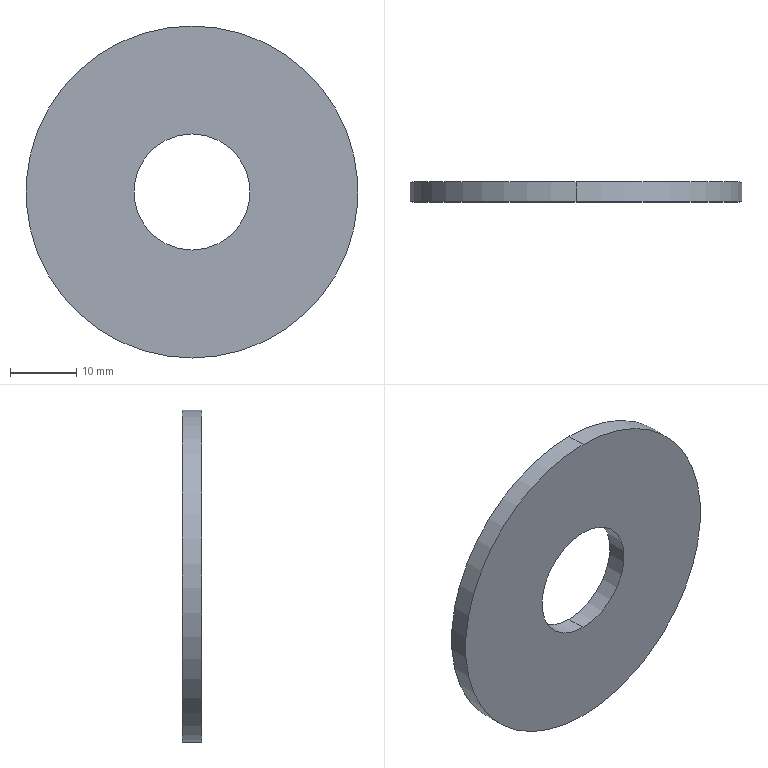Part | SolidWorks | features Extrusion 1 | 1 solid | 6 faces | box 50 x 3 x 50 mm | volume 5169 mm3 | cylinder 4 | plane 2 | commonest cylinder face diameters 17.5 x2 50 x2
STEP:
#1=CARTESIAN_POINT('',(0.,3.,-8.75));
#2=VERTEX_POINT('',#1);
#3=CARTESIAN_POINT('',(0.,3.,8.75));
#4=VERTEX_POINT('',#3);
#5=CARTESIAN_POINT('',(0.,3.,0.));
#6=DIRECTION('',(0.,1.,0.));
#7=DIRECTION('',(0.,0.,1.));
#8=AXIS2_PLACEMENT_3D('',#5,#6,#7);
#9=CIRCLE('',#8,8.75);
#10=EDGE_CURVE('',#2,#4,#9,.T.);
#11=ORIENTED_EDGE('',*,*,#10,.T.);
#12=CARTESIAN_POINT('',(0.,0.,8.75));
#13=VERTEX_POINT('',#12);
#14=CARTESIAN_POINT('',(0.,3.,8.75));
#15=DIRECTION('',(0.,-1.,0.));
#16=VECTOR('',#15,1000.);
#17=LINE('',#14,#16);
#18=EDGE_CURVE('',#4,#13,#17,.T.);
#19=ORIENTED_EDGE('',*,*,#18,.T.);
#20=CARTESIAN_POINT('',(0.,0.,-8.75));
#21=VERTEX_POINT('',#20);
#22=CARTESIAN_POINT('',(0.,0.,0.));
#23=DIRECTION('',(0.,1.,0.));
#24=DIRECTION('',(0.,0.,1.));
#25=AXIS2_PLACEMENT_3D('',#22,#23,#24);
#26=CIRCLE('',#25,8.75);
#27=EDGE_CURVE('',#21,#13,#26,.T.);
#28=ORIENTED_EDGE('',*,*,#27,.F.);
#29=CARTESIAN_POINT('',(0.,3.,-8.75));
#30=DIRECTION('',(0.,-1.,0.));
#31=VECTOR('',#30,1000.);
#32=LINE('',#29,#31);
#33=EDGE_CURVE('',#2,#21,#32,.T.);
#34=ORIENTED_EDGE('',*,*,#33,.F.);
#35=EDGE_LOOP('',(#11,#19,#28,#34));
#36=FACE_OUTER_BOUND('',#35,.T.);
#37=CARTESIAN_POINT('',(0.,3.,0.));
#38=DIRECTION('',(0.,-1.,0.));
#39=DIRECTION('',(0.,0.,-1.));
#40=AXIS2_PLACEMENT_3D('',#37,#38,#39);
#41=CYLINDRICAL_SURFACE('',#40,8.75);
#42=ADVANCED_FACE('',(#36),#41,.F.);
#43=CARTESIAN_POINT('',(0.,3.,25.));
#44=VERTEX_POINT('',#43);
#45=CARTESIAN_POINT('',(0.,3.,-25.));
#46=VERTEX_POINT('',#45);
#47=CARTESIAN_POINT('',(0.,3.,0.));
#48=DIRECTION('',(0.,1.,0.));
#49=DIRECTION('',(0.,0.,1.));
#50=AXIS2_PLACEMENT_3D('',#47,#48,#49);
#51=CIRCLE('',#50,25.);
#52=EDGE_CURVE('',#44,#46,#51,.T.);
#53=ORIENTED_EDGE('',*,*,#52,.F.);
#54=CARTESIAN_POINT('',(0.,0.,25.));
#55=VERTEX_POINT('',#54);
#56=CARTESIAN_POINT('',(0.,3.,25.));
#57=DIRECTION('',(0.,-1.,0.));
#58=VECTOR('',#57,1000.);
#59=LINE('',#56,#58);
#60=EDGE_CURVE('',#44,#55,#59,.T.);
#61=ORIENTED_EDGE('',*,*,#60,.T.);
#62=CARTESIAN_POINT('',(0.,0.,-25.));
#63=VERTEX_POINT('',#62);
#64=CARTESIAN_POINT('',(0.,0.,0.));
#65=DIRECTION('',(0.,1.,0.));
#66=DIRECTION('',(0.,0.,1.));
#67=AXIS2_PLACEMENT_3D('',#64,#65,#66);
#68=CIRCLE('',#67,25.);
#69=EDGE_CURVE('',#55,#63,#68,.T.);
#70=ORIENTED_EDGE('',*,*,#69,.T.);
#71=CARTESIAN_POINT('',(0.,3.,-25.));
#72=DIRECTION('',(0.,-1.,0.));
#73=VECTOR('',#72,1000.);
#74=LINE('',#71,#73);
#75=EDGE_CURVE('',#46,#63,#74,.T.);
#76=ORIENTED_EDGE('',*,*,#75,.F.);
#77=EDGE_LOOP('',(#53,#61,#70,#76));
#78=FACE_OUTER_BOUND('',#77,.T.);
#79=CARTESIAN_POINT('',(0.,3.,0.));
#80=DIRECTION('',(0.,-1.,0.));
#81=DIRECTION('',(0.,0.,-1.));
#82=AXIS2_PLACEMENT_3D('',#79,#80,#81);
#83=CYLINDRICAL_SURFACE('',#82,25.);
#84=ADVANCED_FACE('',(#78),#83,.T.);
#85=CARTESIAN_POINT('',(0.,3.,0.));
#86=DIRECTION('',(0.,1.,0.));
#87=DIRECTION('',(0.,0.,1.));
#88=AXIS2_PLACEMENT_3D('',#85,#86,#87);
#89=CIRCLE('',#88,25.);
#90=EDGE_CURVE('',#46,#44,#89,.T.);
#91=ORIENTED_EDGE('',*,*,#90,.T.);
#92=ORIENTED_EDGE('',*,*,#52,.T.);
#93=EDGE_LOOP('',(#91,#92));
#94=FACE_OUTER_BOUND('',#93,.T.);
#95=ORIENTED_EDGE('',*,*,#10,.F.);
#96=CARTESIAN_POINT('',(0.,3.,0.));
#97=DIRECTION('',(0.,1.,0.));
#98=DIRECTION('',(0.,0.,1.));
#99=AXIS2_PLACEMENT_3D('',#96,#97,#98);
#100=CIRCLE('',#99,8.75);
#101=EDGE_CURVE('',#4,#2,#100,.T.);
#102=ORIENTED_EDGE('',*,*,#101,.F.);
#103=EDGE_LOOP('',(#95,#102));
#104=FACE_BOUND('',#103,.T.);
#105=CARTESIAN_POINT('',(0.,3.,0.));
#106=DIRECTION('',(0.,1.,0.));
#107=DIRECTION('',(0.,0.,1.));
#108=AXIS2_PLACEMENT_3D('',#105,#106,#107);
#109=PLANE('',#108);
#110=ADVANCED_FACE('',(#94,#104),#109,.T.);
#111=CARTESIAN_POINT('',(0.,0.,0.));
#112=DIRECTION('',(0.,1.,0.));
#113=DIRECTION('',(0.,0.,1.));
#114=AXIS2_PLACEMENT_3D('',#111,#112,#113);
#115=CIRCLE('',#114,25.);
#116=EDGE_CURVE('',#63,#55,#115,.T.);
#117=ORIENTED_EDGE('',*,*,#116,.F.);
#118=ORIENTED_EDGE('',*,*,#69,.F.);
#119=EDGE_LOOP('',(#117,#118));
#120=FACE_OUTER_BOUND('',#119,.T.);
#121=ORIENTED_EDGE('',*,*,#27,.T.);
#122=CARTESIAN_POINT('',(0.,0.,0.));
#123=DIRECTION('',(0.,1.,0.));
#124=DIRECTION('',(0.,0.,1.));
#125=AXIS2_PLACEMENT_3D('',#122,#123,#124);
#126=CIRCLE('',#125,8.75);
#127=EDGE_CURVE('',#13,#21,#126,.T.);
#128=ORIENTED_EDGE('',*,*,#127,.T.);
#129=EDGE_LOOP('',(#121,#128));
#130=FACE_BOUND('',#129,.T.);
#131=CARTESIAN_POINT('',(0.,0.,0.));
#132=DIRECTION('',(0.,1.,0.));
#133=DIRECTION('',(0.,0.,1.));
#134=AXIS2_PLACEMENT_3D('',#131,#132,#133);
#135=PLANE('',#134);
#136=ADVANCED_FACE('',(#120,#130),#135,.F.);
#137=ORIENTED_EDGE('',*,*,#60,.F.);
#138=ORIENTED_EDGE('',*,*,#90,.F.);
#139=ORIENTED_EDGE('',*,*,#75,.T.);
#140=ORIENTED_EDGE('',*,*,#116,.T.);
#141=EDGE_LOOP('',(#137,#138,#139,#140));
#142=FACE_OUTER_BOUND('',#141,.T.);
#143=CARTESIAN_POINT('',(0.,3.,0.));
#144=DIRECTION('',(0.,-1.,0.));
#145=DIRECTION('',(0.,0.,-1.));
#146=AXIS2_PLACEMENT_3D('',#143,#144,#145);
#147=CYLINDRICAL_SURFACE('',#146,25.);
#148=ADVANCED_FACE('',(#142),#147,.T.);
#149=ORIENTED_EDGE('',*,*,#18,.F.);
#150=ORIENTED_EDGE('',*,*,#101,.T.);
#151=ORIENTED_EDGE('',*,*,#33,.T.);
#152=ORIENTED_EDGE('',*,*,#127,.F.);
#153=EDGE_LOOP('',(#149,#150,#151,#152));
#154=FACE_OUTER_BOUND('',#153,.T.);
#155=CARTESIAN_POINT('',(0.,3.,0.));
#156=DIRECTION('',(0.,-1.,0.));
#157=DIRECTION('',(0.,0.,-1.));
#158=AXIS2_PLACEMENT_3D('',#155,#156,#157);
#159=CYLINDRICAL_SURFACE('',#158,8.75);
#160=ADVANCED_FACE('',(#154),#159,.F.);
#161=CLOSED_SHELL('',(#42,#84,#110,#136,#148,#160));
#162=MANIFOLD_SOLID_BREP('',#161);
#163=CARTESIAN_POINT('',(0.,0.,0.));
#164=DIRECTION('',(0.,0.,1.));
#165=DIRECTION('',(1.,0.,0.));
#166=AXIS2_PLACEMENT_3D('',#163,#164,#165);
#167=(LENGTH_UNIT()NAMED_UNIT(*)SI_UNIT(.MILLI.,.METRE.));
#168=UNCERTAINTY_MEASURE_WITH_UNIT(LENGTH_MEASURE(0.00001),#167,'','');
#169=(NAMED_UNIT(*)PLANE_ANGLE_UNIT()SI_UNIT($,.RADIAN.));
#170=(NAMED_UNIT(*)SI_UNIT($,.STERADIAN.)SOLID_ANGLE_UNIT());
#171=(GEOMETRIC_REPRESENTATION_CONTEXT(3)GLOBAL_UNCERTAINTY_ASSIGNED_CONTEXT((#168))GLOBAL_UNIT_ASSIGNED_CONTEXT((#167,#169,#170))REPRESENTATION_CONTEXT('',''));
#172=ADVANCED_BREP_SHAPE_REPRESENTATION('',(#162,#166),#171);